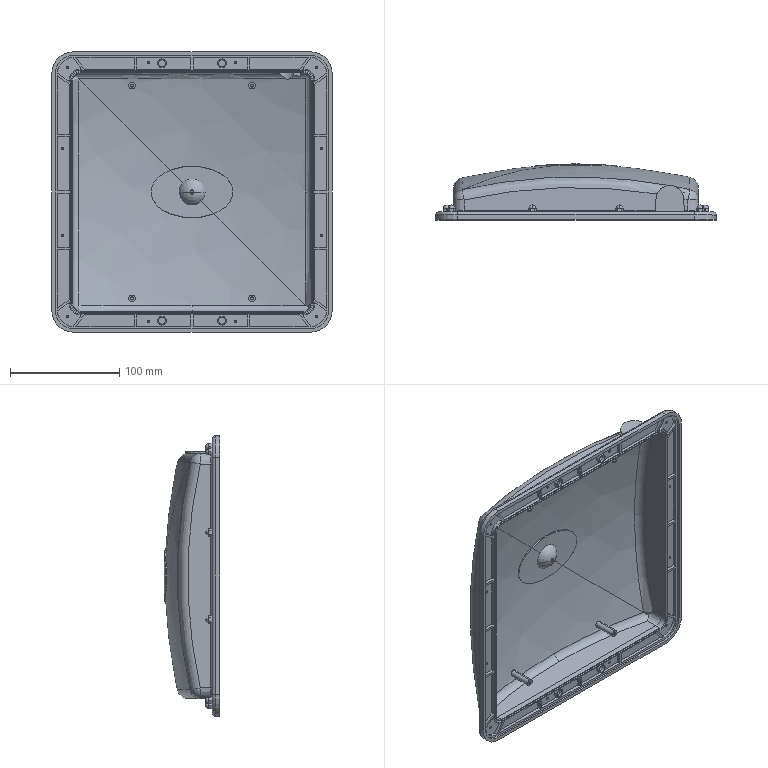Part | SolidWorks | features ICE 12, Fillet 3, Revolution 3, MirrorPattern 2, RevCut 2, 3DProfileFeature 1, CirPattern 1, Extrusion 1, HoleWzd 1, Rib 1, Shell 1, SweepCut 1 | 2 solids | 569 faces | box 257 x 51.2 x 257 mm | volume 287758 mm3 | plane 366 | cylinder 93 | sphere 38 | cone 34 | torus 30 | spline 8 | commonest cylinder face diameters 2.05 x24 6 x12 2.8 x8 6.45 x8 8 x8 3 x5